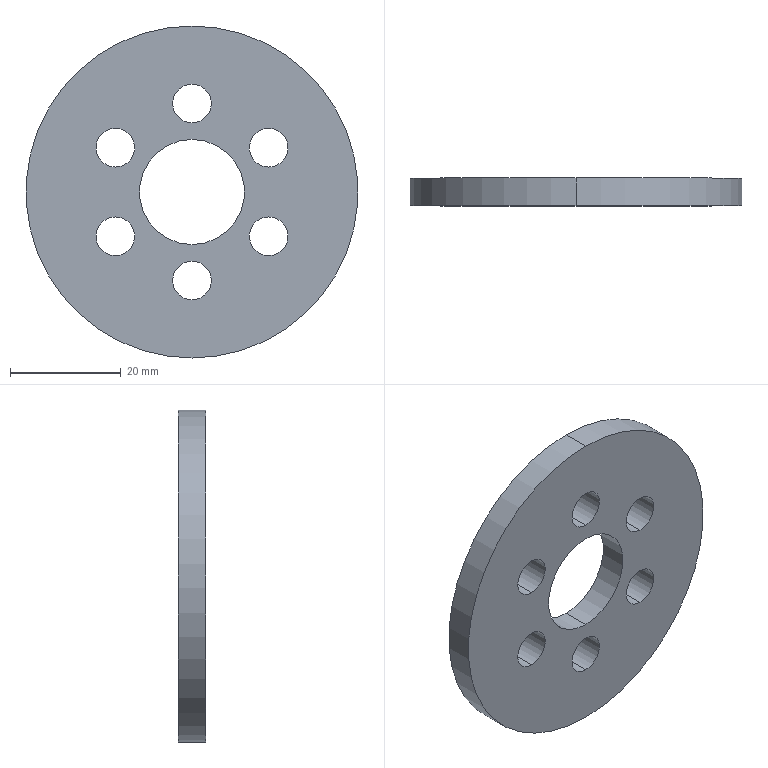Part | 1 solid | 18 faces | box 60 x 5 x 60 mm | volume 11565 mm3 | cylinder 16 | plane 2 | commonest cylinder face diameters 7 x12 19 x2 60 x2
STEP:
#1=CARTESIAN_POINT('',(0.,0.,-19.5));
#2=VERTEX_POINT('',#1);
#3=CARTESIAN_POINT('',(0.,0.,-12.5));
#4=VERTEX_POINT('',#3);
#5=CARTESIAN_POINT('',(0.,0.,-16.));
#6=DIRECTION('',(0.,1.,0.));
#7=DIRECTION('',(0.,0.,1.));
#8=AXIS2_PLACEMENT_3D('',#5,#6,#7);
#9=CIRCLE('',#8,3.5);
#10=EDGE_CURVE('',#2,#4,#9,.T.);
#11=ORIENTED_EDGE('',*,*,#10,.F.);
#12=CARTESIAN_POINT('',(0.,5.,-19.5));
#13=VERTEX_POINT('',#12);
#14=CARTESIAN_POINT('',(0.,5.,-19.5));
#15=DIRECTION('',(0.,1.,0.));
#16=VECTOR('',#15,1000.);
#17=LINE('',#14,#16);
#18=EDGE_CURVE('',#2,#13,#17,.T.);
#19=ORIENTED_EDGE('',*,*,#18,.T.);
#20=CARTESIAN_POINT('',(0.,5.,-12.5));
#21=VERTEX_POINT('',#20);
#22=CARTESIAN_POINT('',(0.,5.,-16.));
#23=DIRECTION('',(0.,1.,0.));
#24=DIRECTION('',(0.,0.,1.));
#25=AXIS2_PLACEMENT_3D('',#22,#23,#24);
#26=CIRCLE('',#25,3.5);
#27=EDGE_CURVE('',#13,#21,#26,.T.);
#28=ORIENTED_EDGE('',*,*,#27,.T.);
#29=CARTESIAN_POINT('',(0.,5.,-12.5));
#30=DIRECTION('',(0.,1.,0.));
#31=VECTOR('',#30,1000.);
#32=LINE('',#29,#31);
#33=EDGE_CURVE('',#4,#21,#32,.T.);
#34=ORIENTED_EDGE('',*,*,#33,.F.);
#35=EDGE_LOOP('',(#11,#19,#28,#34));
#36=FACE_OUTER_BOUND('',#35,.T.);
#37=CARTESIAN_POINT('',(0.,5.,-16.));
#38=DIRECTION('',(0.,1.,0.));
#39=DIRECTION('',(0.,0.,1.));
#40=AXIS2_PLACEMENT_3D('',#37,#38,#39);
#41=CYLINDRICAL_SURFACE('',#40,3.5);
#42=ADVANCED_FACE('',(#36),#41,.F.);
#43=CARTESIAN_POINT('',(13.856,0.,-11.5));
#44=VERTEX_POINT('',#43);
#45=CARTESIAN_POINT('',(13.856,0.,-4.5));
#46=VERTEX_POINT('',#45);
#47=CARTESIAN_POINT('',(13.856,0.,-8.));
#48=DIRECTION('',(0.,1.,0.));
#49=DIRECTION('',(0.,0.,1.));
#50=AXIS2_PLACEMENT_3D('',#47,#48,#49);
#51=CIRCLE('',#50,3.5);
#52=EDGE_CURVE('',#44,#46,#51,.T.);
#53=ORIENTED_EDGE('',*,*,#52,.F.);
#54=CARTESIAN_POINT('',(13.856,5.,-11.5));
#55=VERTEX_POINT('',#54);
#56=CARTESIAN_POINT('',(13.856,5.,-11.5));
#57=DIRECTION('',(0.,1.,0.));
#58=VECTOR('',#57,1000.);
#59=LINE('',#56,#58);
#60=EDGE_CURVE('',#44,#55,#59,.T.);
#61=ORIENTED_EDGE('',*,*,#60,.T.);
#62=CARTESIAN_POINT('',(13.856,5.,-4.5));
#63=VERTEX_POINT('',#62);
#64=CARTESIAN_POINT('',(13.856,5.,-8.));
#65=DIRECTION('',(0.,1.,0.));
#66=DIRECTION('',(0.,0.,1.));
#67=AXIS2_PLACEMENT_3D('',#64,#65,#66);
#68=CIRCLE('',#67,3.5);
#69=EDGE_CURVE('',#55,#63,#68,.T.);
#70=ORIENTED_EDGE('',*,*,#69,.T.);
#71=CARTESIAN_POINT('',(13.856,5.,-4.5));
#72=DIRECTION('',(0.,1.,0.));
#73=VECTOR('',#72,1000.);
#74=LINE('',#71,#73);
#75=EDGE_CURVE('',#46,#63,#74,.T.);
#76=ORIENTED_EDGE('',*,*,#75,.F.);
#77=EDGE_LOOP('',(#53,#61,#70,#76));
#78=FACE_OUTER_BOUND('',#77,.T.);
#79=CARTESIAN_POINT('',(13.856,5.,-8.));
#80=DIRECTION('',(0.,1.,0.));
#81=DIRECTION('',(0.,0.,1.));
#82=AXIS2_PLACEMENT_3D('',#79,#80,#81);
#83=CYLINDRICAL_SURFACE('',#82,3.5);
#84=ADVANCED_FACE('',(#78),#83,.F.);
#85=CARTESIAN_POINT('',(13.856,0.,4.5));
#86=VERTEX_POINT('',#85);
#87=CARTESIAN_POINT('',(13.856,0.,11.5));
#88=VERTEX_POINT('',#87);
#89=CARTESIAN_POINT('',(13.856,0.,8.));
#90=DIRECTION('',(0.,1.,0.));
#91=DIRECTION('',(0.,0.,1.));
#92=AXIS2_PLACEMENT_3D('',#89,#90,#91);
#93=CIRCLE('',#92,3.5);
#94=EDGE_CURVE('',#86,#88,#93,.T.);
#95=ORIENTED_EDGE('',*,*,#94,.F.);
#96=CARTESIAN_POINT('',(13.856,5.,4.5));
#97=VERTEX_POINT('',#96);
#98=CARTESIAN_POINT('',(13.856,5.,4.5));
#99=DIRECTION('',(0.,1.,0.));
#100=VECTOR('',#99,1000.);
#101=LINE('',#98,#100);
#102=EDGE_CURVE('',#86,#97,#101,.T.);
#103=ORIENTED_EDGE('',*,*,#102,.T.);
#104=CARTESIAN_POINT('',(13.856,5.,11.5));
#105=VERTEX_POINT('',#104);
#106=CARTESIAN_POINT('',(13.856,5.,8.));
#107=DIRECTION('',(0.,1.,0.));
#108=DIRECTION('',(0.,0.,1.));
#109=AXIS2_PLACEMENT_3D('',#106,#107,#108);
#110=CIRCLE('',#109,3.5);
#111=EDGE_CURVE('',#97,#105,#110,.T.);
#112=ORIENTED_EDGE('',*,*,#111,.T.);
#113=CARTESIAN_POINT('',(13.856,5.,11.5));
#114=DIRECTION('',(0.,1.,0.));
#115=VECTOR('',#114,1000.);
#116=LINE('',#113,#115);
#117=EDGE_CURVE('',#88,#105,#116,.T.);
#118=ORIENTED_EDGE('',*,*,#117,.F.);
#119=EDGE_LOOP('',(#95,#103,#112,#118));
#120=FACE_OUTER_BOUND('',#119,.T.);
#121=CARTESIAN_POINT('',(13.856,5.,8.));
#122=DIRECTION('',(0.,1.,0.));
#123=DIRECTION('',(0.,0.,1.));
#124=AXIS2_PLACEMENT_3D('',#121,#122,#123);
#125=CYLINDRICAL_SURFACE('',#124,3.5);
#126=ADVANCED_FACE('',(#120),#125,.F.);
#127=CARTESIAN_POINT('',(0.,0.,12.5));
#128=VERTEX_POINT('',#127);
#129=CARTESIAN_POINT('',(0.,0.,19.5));
#130=VERTEX_POINT('',#129);
#131=CARTESIAN_POINT('',(0.,0.,16.));
#132=DIRECTION('',(0.,1.,0.));
#133=DIRECTION('',(0.,0.,1.));
#134=AXIS2_PLACEMENT_3D('',#131,#132,#133);
#135=CIRCLE('',#134,3.5);
#136=EDGE_CURVE('',#128,#130,#135,.T.);
#137=ORIENTED_EDGE('',*,*,#136,.F.);
#138=CARTESIAN_POINT('',(0.,5.,12.5));
#139=VERTEX_POINT('',#138);
#140=CARTESIAN_POINT('',(0.,5.,12.5));
#141=DIRECTION('',(0.,1.,0.));
#142=VECTOR('',#141,1000.);
#143=LINE('',#140,#142);
#144=EDGE_CURVE('',#128,#139,#143,.T.);
#145=ORIENTED_EDGE('',*,*,#144,.T.);
#146=CARTESIAN_POINT('',(0.,5.,19.5));
#147=VERTEX_POINT('',#146);
#148=CARTESIAN_POINT('',(0.,5.,16.));
#149=DIRECTION('',(0.,1.,0.));
#150=DIRECTION('',(0.,0.,1.));
#151=AXIS2_PLACEMENT_3D('',#148,#149,#150);
#152=CIRCLE('',#151,3.5);
#153=EDGE_CURVE('',#139,#147,#152,.T.);
#154=ORIENTED_EDGE('',*,*,#153,.T.);
#155=CARTESIAN_POINT('',(0.,5.,19.5));
#156=DIRECTION('',(0.,1.,0.));
#157=VECTOR('',#156,1000.);
#158=LINE('',#155,#157);
#159=EDGE_CURVE('',#130,#147,#158,.T.);
#160=ORIENTED_EDGE('',*,*,#159,.F.);
#161=EDGE_LOOP('',(#137,#145,#154,#160));
#162=FACE_OUTER_BOUND('',#161,.T.);
#163=CARTESIAN_POINT('',(0.,5.,16.));
#164=DIRECTION('',(0.,1.,0.));
#165=DIRECTION('',(0.,0.,1.));
#166=AXIS2_PLACEMENT_3D('',#163,#164,#165);
#167=CYLINDRICAL_SURFACE('',#166,3.5);
#168=ADVANCED_FACE('',(#162),#167,.F.);
#169=CARTESIAN_POINT('',(-13.856,0.,4.5));
#170=VERTEX_POINT('',#169);
#171=CARTESIAN_POINT('',(-13.856,0.,11.5));
#172=VERTEX_POINT('',#171);
#173=CARTESIAN_POINT('',(-13.856,0.,8.));
#174=DIRECTION('',(0.,1.,0.));
#175=DIRECTION('',(0.,0.,1.));
#176=AXIS2_PLACEMENT_3D('',#173,#174,#175);
#177=CIRCLE('',#176,3.5);
#178=EDGE_CURVE('',#170,#172,#177,.T.);
#179=ORIENTED_EDGE('',*,*,#178,.F.);
#180=CARTESIAN_POINT('',(-13.856,5.,4.5));
#181=VERTEX_POINT('',#180);
#182=CARTESIAN_POINT('',(-13.856,5.,4.5));
#183=DIRECTION('',(0.,1.,0.));
#184=VECTOR('',#183,1000.);
#185=LINE('',#182,#184);
#186=EDGE_CURVE('',#170,#181,#185,.T.);
#187=ORIENTED_EDGE('',*,*,#186,.T.);
#188=CARTESIAN_POINT('',(-13.856,5.,11.5));
#189=VERTEX_POINT('',#188);
#190=CARTESIAN_POINT('',(-13.856,5.,8.));
#191=DIRECTION('',(0.,1.,0.));
#192=DIRECTION('',(0.,0.,1.));
#193=AXIS2_PLACEMENT_3D('',#190,#191,#192);
#194=CIRCLE('',#193,3.5);
#195=EDGE_CURVE('',#181,#189,#194,.T.);
#196=ORIENTED_EDGE('',*,*,#195,.T.);
#197=CARTESIAN_POINT('',(-13.856,5.,11.5));
#198=DIRECTION('',(0.,1.,0.));
#199=VECTOR('',#198,1000.);
#200=LINE('',#197,#199);
#201=EDGE_CURVE('',#172,#189,#200,.T.);
#202=ORIENTED_EDGE('',*,*,#201,.F.);
#203=EDGE_LOOP('',(#179,#187,#196,#202));
#204=FACE_OUTER_BOUND('',#203,.T.);
#205=CARTESIAN_POINT('',(-13.856,5.,8.));
#206=DIRECTION('',(0.,1.,0.));
#207=DIRECTION('',(0.,0.,1.));
#208=AXIS2_PLACEMENT_3D('',#205,#206,#207);
#209=CYLINDRICAL_SURFACE('',#208,3.5);
#210=ADVANCED_FACE('',(#204),#209,.F.);
#211=CARTESIAN_POINT('',(-13.856,0.,-11.5));
#212=VERTEX_POINT('',#211);
#213=CARTESIAN_POINT('',(-13.856,0.,-4.5));
#214=VERTEX_POINT('',#213);
#215=CARTESIAN_POINT('',(-13.856,0.,-8.));
#216=DIRECTION('',(0.,1.,0.));
#217=DIRECTION('',(0.,0.,1.));
#218=AXIS2_PLACEMENT_3D('',#215,#216,#217);
#219=CIRCLE('',#218,3.5);
#220=EDGE_CURVE('',#212,#214,#219,.T.);
#221=ORIENTED_EDGE('',*,*,#220,.F.);
#222=CARTESIAN_POINT('',(-13.856,5.,-11.5));
#223=VERTEX_POINT('',#222);
#224=CARTESIAN_POINT('',(-13.856,5.,-11.5));
#225=DIRECTION('',(0.,1.,0.));
#226=VECTOR('',#225,1000.);
#227=LINE('',#224,#226);
#228=EDGE_CURVE('',#212,#223,#227,.T.);
#229=ORIENTED_EDGE('',*,*,#228,.T.);
#230=CARTESIAN_POINT('',(-13.856,5.,-4.5));
#231=VERTEX_POINT('',#230);
#232=CARTESIAN_POINT('',(-13.856,5.,-8.));
#233=DIRECTION('',(0.,1.,0.));
#234=DIRECTION('',(0.,0.,1.));
#235=AXIS2_PLACEMENT_3D('',#232,#233,#234);
#236=CIRCLE('',#235,3.5);
#237=EDGE_CURVE('',#223,#231,#236,.T.);
#238=ORIENTED_EDGE('',*,*,#237,.T.);
#239=CARTESIAN_POINT('',(-13.856,5.,-4.5));
#240=DIRECTION('',(0.,1.,0.));
#241=VECTOR('',#240,1000.);
#242=LINE('',#239,#241);
#243=EDGE_CURVE('',#214,#231,#242,.T.);
#244=ORIENTED_EDGE('',*,*,#243,.F.);
#245=EDGE_LOOP('',(#221,#229,#238,#244));
#246=FACE_OUTER_BOUND('',#245,.T.);
#247=CARTESIAN_POINT('',(-13.856,5.,-8.));
#248=DIRECTION('',(0.,1.,0.));
#249=DIRECTION('',(0.,0.,1.));
#250=AXIS2_PLACEMENT_3D('',#247,#248,#249);
#251=CYLINDRICAL_SURFACE('',#250,3.5);
#252=ADVANCED_FACE('',(#246),#251,.F.);
#253=CARTESIAN_POINT('',(0.,5.,-9.5));
#254=VERTEX_POINT('',#253);
#255=CARTESIAN_POINT('',(0.,5.,9.5));
#256=VERTEX_POINT('',#255);
#257=CARTESIAN_POINT('',(0.,5.,0.));
#258=DIRECTION('',(0.,1.,0.));
#259=DIRECTION('',(0.,0.,1.));
#260=AXIS2_PLACEMENT_3D('',#257,#258,#259);
#261=CIRCLE('',#260,9.5);
#262=EDGE_CURVE('',#254,#256,#261,.T.);
#263=ORIENTED_EDGE('',*,*,#262,.T.);
#264=CARTESIAN_POINT('',(0.,0.,9.5));
#265=VERTEX_POINT('',#264);
#266=CARTESIAN_POINT('',(0.,5.,9.5));
#267=DIRECTION('',(0.,-1.,0.));
#268=VECTOR('',#267,1000.);
#269=LINE('',#266,#268);
#270=EDGE_CURVE('',#256,#265,#269,.T.);
#271=ORIENTED_EDGE('',*,*,#270,.T.);
#272=CARTESIAN_POINT('',(0.,0.,-9.5));
#273=VERTEX_POINT('',#272);
#274=CARTESIAN_POINT('',(0.,0.,0.));
#275=DIRECTION('',(0.,1.,0.));
#276=DIRECTION('',(0.,0.,1.));
#277=AXIS2_PLACEMENT_3D('',#274,#275,#276);
#278=CIRCLE('',#277,9.5);
#279=EDGE_CURVE('',#273,#265,#278,.T.);
#280=ORIENTED_EDGE('',*,*,#279,.F.);
#281=CARTESIAN_POINT('',(0.,5.,-9.5));
#282=DIRECTION('',(0.,-1.,0.));
#283=VECTOR('',#282,1000.);
#284=LINE('',#281,#283);
#285=EDGE_CURVE('',#254,#273,#284,.T.);
#286=ORIENTED_EDGE('',*,*,#285,.F.);
#287=EDGE_LOOP('',(#263,#271,#280,#286));
#288=FACE_OUTER_BOUND('',#287,.T.);
#289=CARTESIAN_POINT('',(0.,5.,0.));
#290=DIRECTION('',(0.,-1.,0.));
#291=DIRECTION('',(0.,0.,-1.));
#292=AXIS2_PLACEMENT_3D('',#289,#290,#291);
#293=CYLINDRICAL_SURFACE('',#292,9.5);
#294=ADVANCED_FACE('',(#288),#293,.F.);
#295=CARTESIAN_POINT('',(0.,5.,30.));
#296=VERTEX_POINT('',#295);
#297=CARTESIAN_POINT('',(0.,5.,-30.));
#298=VERTEX_POINT('',#297);
#299=CARTESIAN_POINT('',(0.,5.,0.));
#300=DIRECTION('',(0.,1.,0.));
#301=DIRECTION('',(0.,0.,1.));
#302=AXIS2_PLACEMENT_3D('',#299,#300,#301);
#303=CIRCLE('',#302,30.);
#304=EDGE_CURVE('',#296,#298,#303,.T.);
#305=ORIENTED_EDGE('',*,*,#304,.F.);
#306=CARTESIAN_POINT('',(0.,0.,30.));
#307=VERTEX_POINT('',#306);
#308=CARTESIAN_POINT('',(0.,5.,30.));
#309=DIRECTION('',(0.,-1.,0.));
#310=VECTOR('',#309,1000.);
#311=LINE('',#308,#310);
#312=EDGE_CURVE('',#296,#307,#311,.T.);
#313=ORIENTED_EDGE('',*,*,#312,.T.);
#314=CARTESIAN_POINT('',(0.,0.,-30.));
#315=VERTEX_POINT('',#314);
#316=CARTESIAN_POINT('',(0.,0.,0.));
#317=DIRECTION('',(0.,1.,0.));
#318=DIRECTION('',(0.,0.,1.));
#319=AXIS2_PLACEMENT_3D('',#316,#317,#318);
#320=CIRCLE('',#319,30.);
#321=EDGE_CURVE('',#307,#315,#320,.T.);
#322=ORIENTED_EDGE('',*,*,#321,.T.);
#323=CARTESIAN_POINT('',(0.,5.,-30.));
#324=DIRECTION('',(0.,-1.,0.));
#325=VECTOR('',#324,1000.);
#326=LINE('',#323,#325);
#327=EDGE_CURVE('',#298,#315,#326,.T.);
#328=ORIENTED_EDGE('',*,*,#327,.F.);
#329=EDGE_LOOP('',(#305,#313,#322,#328));
#330=FACE_OUTER_BOUND('',#329,.T.);
#331=CARTESIAN_POINT('',(0.,5.,0.));
#332=DIRECTION('',(0.,-1.,0.));
#333=DIRECTION('',(0.,0.,-1.));
#334=AXIS2_PLACEMENT_3D('',#331,#332,#333);
#335=CYLINDRICAL_SURFACE('',#334,30.);
#336=ADVANCED_FACE('',(#330),#335,.T.);
#337=CARTESIAN_POINT('',(0.,5.,-16.));
#338=DIRECTION('',(0.,1.,0.));
#339=DIRECTION('',(0.,0.,1.));
#340=AXIS2_PLACEMENT_3D('',#337,#338,#339);
#341=CIRCLE('',#340,3.5);
#342=EDGE_CURVE('',#21,#13,#341,.T.);
#343=ORIENTED_EDGE('',*,*,#342,.F.);
#344=ORIENTED_EDGE('',*,*,#27,.F.);
#345=EDGE_LOOP('',(#343,#344));
#346=FACE_BOUND('',#345,.T.);
#347=CARTESIAN_POINT('',(13.856,5.,-8.));
#348=DIRECTION('',(0.,1.,0.));
#349=DIRECTION('',(0.,0.,1.));
#350=AXIS2_PLACEMENT_3D('',#347,#348,#349);
#351=CIRCLE('',#350,3.5);
#352=EDGE_CURVE('',#63,#55,#351,.T.);
#353=ORIENTED_EDGE('',*,*,#352,.F.);
#354=ORIENTED_EDGE('',*,*,#69,.F.);
#355=EDGE_LOOP('',(#353,#354));
#356=FACE_BOUND('',#355,.T.);
#357=CARTESIAN_POINT('',(13.856,5.,8.));
#358=DIRECTION('',(0.,1.,0.));
#359=DIRECTION('',(0.,0.,1.));
#360=AXIS2_PLACEMENT_3D('',#357,#358,#359);
#361=CIRCLE('',#360,3.5);
#362=EDGE_CURVE('',#105,#97,#361,.T.);
#363=ORIENTED_EDGE('',*,*,#362,.F.);
#364=ORIENTED_EDGE('',*,*,#111,.F.);
#365=EDGE_LOOP('',(#363,#364));
#366=FACE_BOUND('',#365,.T.);
#367=CARTESIAN_POINT('',(0.,5.,16.));
#368=DIRECTION('',(0.,1.,0.));
#369=DIRECTION('',(0.,0.,1.));
#370=AXIS2_PLACEMENT_3D('',#367,#368,#369);
#371=CIRCLE('',#370,3.5);
#372=EDGE_CURVE('',#147,#139,#371,.T.);
#373=ORIENTED_EDGE('',*,*,#372,.F.);
#374=ORIENTED_EDGE('',*,*,#153,.F.);
#375=EDGE_LOOP('',(#373,#374));
#376=FACE_BOUND('',#375,.T.);
#377=CARTESIAN_POINT('',(-13.856,5.,8.));
#378=DIRECTION('',(0.,1.,0.));
#379=DIRECTION('',(0.,0.,1.));
#380=AXIS2_PLACEMENT_3D('',#377,#378,#379);
#381=CIRCLE('',#380,3.5);
#382=EDGE_CURVE('',#189,#181,#381,.T.);
#383=ORIENTED_EDGE('',*,*,#382,.F.);
#384=ORIENTED_EDGE('',*,*,#195,.F.);
#385=EDGE_LOOP('',(#383,#384));
#386=FACE_BOUND('',#385,.T.);
#387=CARTESIAN_POINT('',(-13.856,5.,-8.));
#388=DIRECTION('',(0.,1.,0.));
#389=DIRECTION('',(0.,0.,1.));
#390=AXIS2_PLACEMENT_3D('',#387,#388,#389);
#391=CIRCLE('',#390,3.5);
#392=EDGE_CURVE('',#231,#223,#391,.T.);
#393=ORIENTED_EDGE('',*,*,#392,.F.);
#394=ORIENTED_EDGE('',*,*,#237,.F.);
#395=EDGE_LOOP('',(#393,#394));
#396=FACE_BOUND('',#395,.T.);
#397=CARTESIAN_POINT('',(0.,5.,0.));
#398=DIRECTION('',(0.,1.,0.));
#399=DIRECTION('',(0.,0.,1.));
#400=AXIS2_PLACEMENT_3D('',#397,#398,#399);
#401=CIRCLE('',#400,30.);
#402=EDGE_CURVE('',#298,#296,#401,.T.);
#403=ORIENTED_EDGE('',*,*,#402,.T.);
#404=ORIENTED_EDGE('',*,*,#304,.T.);
#405=EDGE_LOOP('',(#403,#404));
#406=FACE_OUTER_BOUND('',#405,.T.);
#407=ORIENTED_EDGE('',*,*,#262,.F.);
#408=CARTESIAN_POINT('',(0.,5.,0.));
#409=DIRECTION('',(0.,1.,0.));
#410=DIRECTION('',(0.,0.,1.));
#411=AXIS2_PLACEMENT_3D('',#408,#409,#410);
#412=CIRCLE('',#411,9.5);
#413=EDGE_CURVE('',#256,#254,#412,.T.);
#414=ORIENTED_EDGE('',*,*,#413,.F.);
#415=EDGE_LOOP('',(#407,#414));
#416=FACE_BOUND('',#415,.T.);
#417=CARTESIAN_POINT('',(0.,5.,0.));
#418=DIRECTION('',(0.,1.,0.));
#419=DIRECTION('',(0.,0.,1.));
#420=AXIS2_PLACEMENT_3D('',#417,#418,#419);
#421=PLANE('',#420);
#422=ADVANCED_FACE('',(#346,#356,#366,#376,#386,#396,#406,#416),#421,.T.);
#423=CARTESIAN_POINT('',(0.,0.,-16.));
#424=DIRECTION('',(0.,1.,0.));
#425=DIRECTION('',(0.,0.,1.));
#426=AXIS2_PLACEMENT_3D('',#423,#424,#425);
#427=CIRCLE('',#426,3.5);
#428=EDGE_CURVE('',#4,#2,#427,.T.);
#429=ORIENTED_EDGE('',*,*,#428,.T.);
#430=ORIENTED_EDGE('',*,*,#10,.T.);
#431=EDGE_LOOP('',(#429,#430));
#432=FACE_BOUND('',#431,.T.);
#433=CARTESIAN_POINT('',(13.856,0.,-8.));
#434=DIRECTION('',(0.,1.,0.));
#435=DIRECTION('',(0.,0.,1.));
#436=AXIS2_PLACEMENT_3D('',#433,#434,#435);
#437=CIRCLE('',#436,3.5);
#438=EDGE_CURVE('',#46,#44,#437,.T.);
#439=ORIENTED_EDGE('',*,*,#438,.T.);
#440=ORIENTED_EDGE('',*,*,#52,.T.);
#441=EDGE_LOOP('',(#439,#440));
#442=FACE_BOUND('',#441,.T.);
#443=CARTESIAN_POINT('',(13.856,0.,8.));
#444=DIRECTION('',(0.,1.,0.));
#445=DIRECTION('',(0.,0.,1.));
#446=AXIS2_PLACEMENT_3D('',#443,#444,#445);
#447=CIRCLE('',#446,3.5);
#448=EDGE_CURVE('',#88,#86,#447,.T.);
#449=ORIENTED_EDGE('',*,*,#448,.T.);
#450=ORIENTED_EDGE('',*,*,#94,.T.);
#451=EDGE_LOOP('',(#449,#450));
#452=FACE_BOUND('',#451,.T.);
#453=CARTESIAN_POINT('',(0.,0.,16.));
#454=DIRECTION('',(0.,1.,0.));
#455=DIRECTION('',(0.,0.,1.));
#456=AXIS2_PLACEMENT_3D('',#453,#454,#455);
#457=CIRCLE('',#456,3.5);
#458=EDGE_CURVE('',#130,#128,#457,.T.);
#459=ORIENTED_EDGE('',*,*,#458,.T.);
#460=ORIENTED_EDGE('',*,*,#136,.T.);
#461=EDGE_LOOP('',(#459,#460));
#462=FACE_BOUND('',#461,.T.);
#463=CARTESIAN_POINT('',(-13.856,0.,8.));
#464=DIRECTION('',(0.,1.,0.));
#465=DIRECTION('',(0.,0.,1.));
#466=AXIS2_PLACEMENT_3D('',#463,#464,#465);
#467=CIRCLE('',#466,3.5);
#468=EDGE_CURVE('',#172,#170,#467,.T.);
#469=ORIENTED_EDGE('',*,*,#468,.T.);
#470=ORIENTED_EDGE('',*,*,#178,.T.);
#471=EDGE_LOOP('',(#469,#470));
#472=FACE_BOUND('',#471,.T.);
#473=CARTESIAN_POINT('',(-13.856,0.,-8.));
#474=DIRECTION('',(0.,1.,0.));
#475=DIRECTION('',(0.,0.,1.));
#476=AXIS2_PLACEMENT_3D('',#473,#474,#475);
#477=CIRCLE('',#476,3.5);
#478=EDGE_CURVE('',#214,#212,#477,.T.);
#479=ORIENTED_EDGE('',*,*,#478,.T.);
#480=ORIENTED_EDGE('',*,*,#220,.T.);
#481=EDGE_LOOP('',(#479,#480));
#482=FACE_BOUND('',#481,.T.);
#483=CARTESIAN_POINT('',(0.,0.,0.));
#484=DIRECTION('',(0.,1.,0.));
#485=DIRECTION('',(0.,0.,1.));
#486=AXIS2_PLACEMENT_3D('',#483,#484,#485);
#487=CIRCLE('',#486,30.);
#488=EDGE_CURVE('',#315,#307,#487,.T.);
#489=ORIENTED_EDGE('',*,*,#488,.F.);
#490=ORIENTED_EDGE('',*,*,#321,.F.);
#491=EDGE_LOOP('',(#489,#490));
#492=FACE_OUTER_BOUND('',#491,.T.);
#493=ORIENTED_EDGE('',*,*,#279,.T.);
#494=CARTESIAN_POINT('',(0.,0.,0.));
#495=DIRECTION('',(0.,1.,0.));
#496=DIRECTION('',(0.,0.,1.));
#497=AXIS2_PLACEMENT_3D('',#494,#495,#496);
#498=CIRCLE('',#497,9.5);
#499=EDGE_CURVE('',#265,#273,#498,.T.);
#500=ORIENTED_EDGE('',*,*,#499,.T.);
#501=EDGE_LOOP('',(#493,#500));
#502=FACE_BOUND('',#501,.T.);
#503=CARTESIAN_POINT('',(0.,0.,0.));
#504=DIRECTION('',(0.,1.,0.));
#505=DIRECTION('',(0.,0.,1.));
#506=AXIS2_PLACEMENT_3D('',#503,#504,#505);
#507=PLANE('',#506);
#508=ADVANCED_FACE('',(#432,#442,#452,#462,#472,#482,#492,#502),#507,.F.);
#509=ORIENTED_EDGE('',*,*,#312,.F.);
#510=ORIENTED_EDGE('',*,*,#402,.F.);
#511=ORIENTED_EDGE('',*,*,#327,.T.);
#512=ORIENTED_EDGE('',*,*,#488,.T.);
#513=EDGE_LOOP('',(#509,#510,#511,#512));
#514=FACE_OUTER_BOUND('',#513,.T.);
#515=CARTESIAN_POINT('',(0.,5.,0.));
#516=DIRECTION('',(0.,-1.,0.));
#517=DIRECTION('',(0.,0.,-1.));
#518=AXIS2_PLACEMENT_3D('',#515,#516,#517);
#519=CYLINDRICAL_SURFACE('',#518,30.);
#520=ADVANCED_FACE('',(#514),#519,.T.);
#521=ORIENTED_EDGE('',*,*,#270,.F.);
#522=ORIENTED_EDGE('',*,*,#413,.T.);
#523=ORIENTED_EDGE('',*,*,#285,.T.);
#524=ORIENTED_EDGE('',*,*,#499,.F.);
#525=EDGE_LOOP('',(#521,#522,#523,#524));
#526=FACE_OUTER_BOUND('',#525,.T.);
#527=CARTESIAN_POINT('',(0.,5.,0.));
#528=DIRECTION('',(0.,-1.,0.));
#529=DIRECTION('',(0.,0.,-1.));
#530=AXIS2_PLACEMENT_3D('',#527,#528,#529);
#531=CYLINDRICAL_SURFACE('',#530,9.5);
#532=ADVANCED_FACE('',(#526),#531,.F.);
#533=ORIENTED_EDGE('',*,*,#228,.F.);
#534=ORIENTED_EDGE('',*,*,#478,.F.);
#535=ORIENTED_EDGE('',*,*,#243,.T.);
#536=ORIENTED_EDGE('',*,*,#392,.T.);
#537=EDGE_LOOP('',(#533,#534,#535,#536));
#538=FACE_OUTER_BOUND('',#537,.T.);
#539=CARTESIAN_POINT('',(-13.856,5.,-8.));
#540=DIRECTION('',(0.,1.,0.));
#541=DIRECTION('',(0.,0.,1.));
#542=AXIS2_PLACEMENT_3D('',#539,#540,#541);
#543=CYLINDRICAL_SURFACE('',#542,3.5);
#544=ADVANCED_FACE('',(#538),#543,.F.);
#545=ORIENTED_EDGE('',*,*,#186,.F.);
#546=ORIENTED_EDGE('',*,*,#468,.F.);
#547=ORIENTED_EDGE('',*,*,#201,.T.);
#548=ORIENTED_EDGE('',*,*,#382,.T.);
#549=EDGE_LOOP('',(#545,#546,#547,#548));
#550=FACE_OUTER_BOUND('',#549,.T.);
#551=CARTESIAN_POINT('',(-13.856,5.,8.));
#552=DIRECTION('',(0.,1.,0.));
#553=DIRECTION('',(0.,0.,1.));
#554=AXIS2_PLACEMENT_3D('',#551,#552,#553);
#555=CYLINDRICAL_SURFACE('',#554,3.5);
#556=ADVANCED_FACE('',(#550),#555,.F.);
#557=ORIENTED_EDGE('',*,*,#144,.F.);
#558=ORIENTED_EDGE('',*,*,#458,.F.);
#559=ORIENTED_EDGE('',*,*,#159,.T.);
#560=ORIENTED_EDGE('',*,*,#372,.T.);
#561=EDGE_LOOP('',(#557,#558,#559,#560));
#562=FACE_OUTER_BOUND('',#561,.T.);
#563=CARTESIAN_POINT('',(0.,5.,16.));
#564=DIRECTION('',(0.,1.,0.));
#565=DIRECTION('',(0.,0.,1.));
#566=AXIS2_PLACEMENT_3D('',#563,#564,#565);
#567=CYLINDRICAL_SURFACE('',#566,3.5);
#568=ADVANCED_FACE('',(#562),#567,.F.);
#569=ORIENTED_EDGE('',*,*,#102,.F.);
#570=ORIENTED_EDGE('',*,*,#448,.F.);
#571=ORIENTED_EDGE('',*,*,#117,.T.);
#572=ORIENTED_EDGE('',*,*,#362,.T.);
#573=EDGE_LOOP('',(#569,#570,#571,#572));
#574=FACE_OUTER_BOUND('',#573,.T.);
#575=CARTESIAN_POINT('',(13.856,5.,8.));
#576=DIRECTION('',(0.,1.,0.));
#577=DIRECTION('',(0.,0.,1.));
#578=AXIS2_PLACEMENT_3D('',#575,#576,#577);
#579=CYLINDRICAL_SURFACE('',#578,3.5);
#580=ADVANCED_FACE('',(#574),#579,.F.);
#581=ORIENTED_EDGE('',*,*,#60,.F.);
#582=ORIENTED_EDGE('',*,*,#438,.F.);
#583=ORIENTED_EDGE('',*,*,#75,.T.);
#584=ORIENTED_EDGE('',*,*,#352,.T.);
#585=EDGE_LOOP('',(#581,#582,#583,#584));
#586=FACE_OUTER_BOUND('',#585,.T.);
#587=CARTESIAN_POINT('',(13.856,5.,-8.));
#588=DIRECTION('',(0.,1.,0.));
#589=DIRECTION('',(0.,0.,1.));
#590=AXIS2_PLACEMENT_3D('',#587,#588,#589);
#591=CYLINDRICAL_SURFACE('',#590,3.5);
#592=ADVANCED_FACE('',(#586),#591,.F.);
#593=ORIENTED_EDGE('',*,*,#18,.F.);
#594=ORIENTED_EDGE('',*,*,#428,.F.);
#595=ORIENTED_EDGE('',*,*,#33,.T.);
#596=ORIENTED_EDGE('',*,*,#342,.T.);
#597=EDGE_LOOP('',(#593,#594,#595,#596));
#598=FACE_OUTER_BOUND('',#597,.T.);
#599=CARTESIAN_POINT('',(0.,5.,-16.));
#600=DIRECTION('',(0.,1.,0.));
#601=DIRECTION('',(0.,0.,1.));
#602=AXIS2_PLACEMENT_3D('',#599,#600,#601);
#603=CYLINDRICAL_SURFACE('',#602,3.5);
#604=ADVANCED_FACE('',(#598),#603,.F.);
#605=CLOSED_SHELL('',(#42,#84,#126,#168,#210,#252,#294,#336,#422,#508,#520,#532,#544,#556,#568,#580,#592,#604));
#606=MANIFOLD_SOLID_BREP('',#605);
#607=CARTESIAN_POINT('',(0.,0.,0.));
#608=DIRECTION('',(0.,0.,1.));
#609=DIRECTION('',(1.,0.,0.));
#610=AXIS2_PLACEMENT_3D('',#607,#608,#609);
#611=(LENGTH_UNIT()NAMED_UNIT(*)SI_UNIT(.MILLI.,.METRE.));
#612=UNCERTAINTY_MEASURE_WITH_UNIT(LENGTH_MEASURE(0.00001),#611,'','');
#613=(NAMED_UNIT(*)PLANE_ANGLE_UNIT()SI_UNIT($,.RADIAN.));
#614=(NAMED_UNIT(*)SI_UNIT($,.STERADIAN.)SOLID_ANGLE_UNIT());
#615=(GEOMETRIC_REPRESENTATION_CONTEXT(3)GLOBAL_UNCERTAINTY_ASSIGNED_CONTEXT((#612))GLOBAL_UNIT_ASSIGNED_CONTEXT((#611,#613,#614))REPRESENTATION_CONTEXT('',''));
#616=ADVANCED_BREP_SHAPE_REPRESENTATION('',(#606,#610),#615);